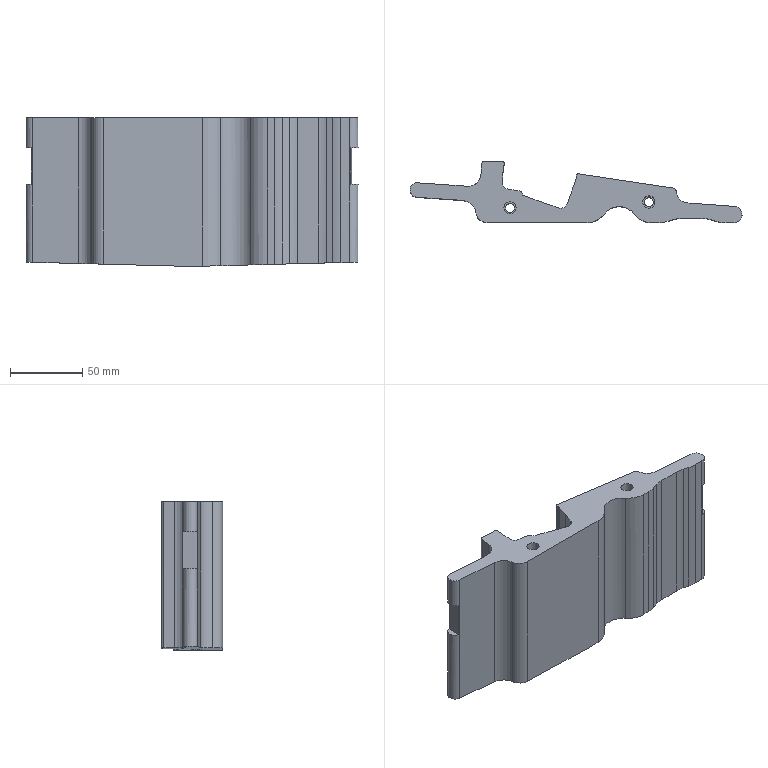Part | NX | features 8 2 | 1 solid | 65 faces | box 229.659 x 42.553 x 103 mm | volume 425610 mm3 | plane 36 | cylinder 29 | commonest cylinder face diameters 2 x6 40 x4 4 x2 6.2 x2 8.5 x2 10 x2